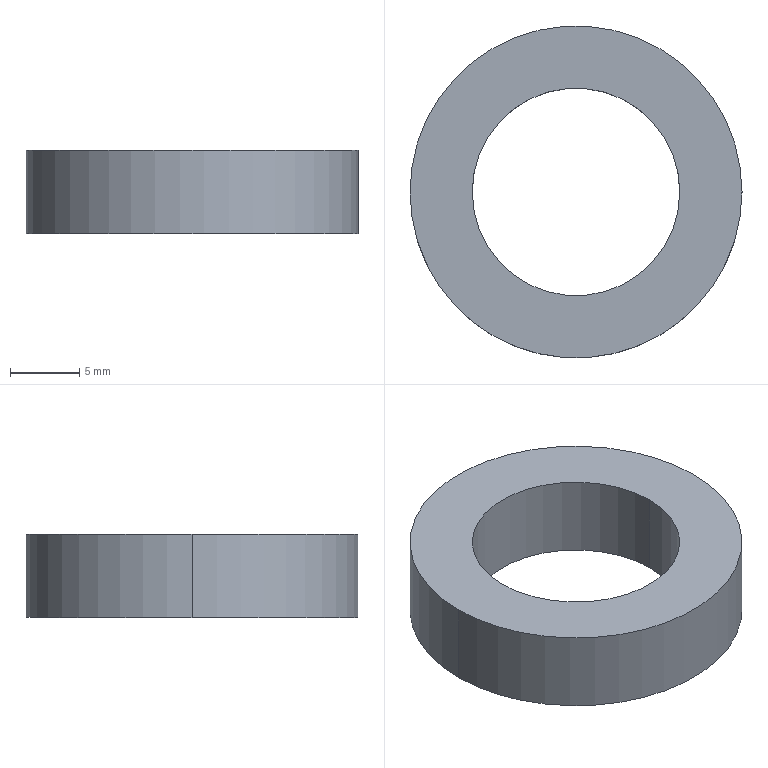Part | STEP file | PN_0016 (stop plate) | 1 solid | 6 faces | box 24 x 24 x 6 mm | volume 1654 mm3 | cylinder 4 | plane 2 | commonest cylinder face diameters 15 x2 24 x2
STEP:
#1=CARTESIAN_POINT('',(0.,0.,0.));
#2=DIRECTION('',(0.,0.,1.));
#3=DIRECTION('',(1.,0.,0.));
#4=AXIS2_PLACEMENT_3D('',#1,#2,#3);
#5=CARTESIAN_POINT('',(-7.5,0.,6.));
#6=VERTEX_POINT('',#5);
#7=CARTESIAN_POINT('',(-7.5,0.,0.));
#8=VERTEX_POINT('',#7);
#9=CARTESIAN_POINT('',(-7.5,0.,6.));
#10=DIRECTION('',(0.,0.,-1.));
#11=VECTOR('',#10,1.);
#12=LINE('',#9,#11);
#13=CARTESIAN_POINT('',(0.,0.,6.));
#14=DIRECTION('',(0.,0.,-1.));
#15=DIRECTION('',(-1.,0.,0.));
#16=AXIS2_PLACEMENT_3D('',#13,#14,#15);
#17=CYLINDRICAL_SURFACE('',#16,7.5);
#18=CARTESIAN_POINT('',(6.283,0.));
#19=DIRECTION('',(0.,1.));
#20=VECTOR('',#19,1.);
#21=LINE('',#18,#20);
#22=(GEOMETRIC_REPRESENTATION_CONTEXT(2)PARAMETRIC_REPRESENTATION_CONTEXT()REPRESENTATION_CONTEXT('',''));
#23=DEFINITIONAL_REPRESENTATION('',(#21),#22);
#24=PCURVE('',#17,#23);
#25=CARTESIAN_POINT('',(0.,0.,6.));
#26=DIRECTION('',(0.,0.,-1.));
#27=DIRECTION('',(-1.,0.,0.));
#28=AXIS2_PLACEMENT_3D('',#25,#26,#27);
#29=CYLINDRICAL_SURFACE('',#28,7.5);
#30=CARTESIAN_POINT('',(0.,0.));
#31=DIRECTION('',(0.,1.));
#32=VECTOR('',#31,1.);
#33=LINE('',#30,#32);
#34=(GEOMETRIC_REPRESENTATION_CONTEXT(2)PARAMETRIC_REPRESENTATION_CONTEXT()REPRESENTATION_CONTEXT('',''));
#35=DEFINITIONAL_REPRESENTATION('',(#33),#34);
#36=PCURVE('',#29,#35);
#37=SURFACE_CURVE('',#12,(#24,#36),.PCURVE_S1.);
#38=EDGE_CURVE('',#6,#8,#37,.T.);
#39=ORIENTED_EDGE('',*,*,#38,.T.);
#40=CARTESIAN_POINT('',(7.5,0.,0.));
#41=VERTEX_POINT('',#40);
#42=CARTESIAN_POINT('',(0.,0.,0.));
#43=DIRECTION('',(0.,0.,1.));
#44=DIRECTION('',(1.,0.,0.));
#45=AXIS2_PLACEMENT_3D('',#42,#43,#44);
#46=CIRCLE('',#45,7.5);
#47=CARTESIAN_POINT('',(9.425,6.));
#48=DIRECTION('',(-1.,0.));
#49=VECTOR('',#48,1.);
#50=LINE('',#47,#49);
#51=(GEOMETRIC_REPRESENTATION_CONTEXT(2)PARAMETRIC_REPRESENTATION_CONTEXT()REPRESENTATION_CONTEXT('',''));
#52=DEFINITIONAL_REPRESENTATION('',(#50),#51);
#53=PCURVE('',#17,#52);
#54=CARTESIAN_POINT('',(0.,0.,0.));
#55=DIRECTION('',(0.,0.,1.));
#56=DIRECTION('',(1.,0.,0.));
#57=AXIS2_PLACEMENT_3D('',#54,#55,#56);
#58=PLANE('',#57);
#59=CARTESIAN_POINT('',(0.,0.));
#60=DIRECTION('',(1.,0.));
#61=AXIS2_PLACEMENT_2D('',#59,#60);
#62=CIRCLE('',#61,7.5);
#63=(GEOMETRIC_REPRESENTATION_CONTEXT(2)PARAMETRIC_REPRESENTATION_CONTEXT()REPRESENTATION_CONTEXT('',''));
#64=DEFINITIONAL_REPRESENTATION('',(#62),#63);
#65=PCURVE('',#58,#64);
#66=SURFACE_CURVE('',#46,(#53,#65),.PCURVE_S1.);
#67=EDGE_CURVE('',#8,#41,#66,.T.);
#68=ORIENTED_EDGE('',*,*,#67,.T.);
#69=CARTESIAN_POINT('',(7.5,0.,6.));
#70=VERTEX_POINT('',#69);
#71=CARTESIAN_POINT('',(7.5,0.,6.));
#72=DIRECTION('',(0.,0.,-1.));
#73=VECTOR('',#72,1.);
#74=LINE('',#71,#73);
#75=CARTESIAN_POINT('',(3.142,0.));
#76=DIRECTION('',(0.,1.));
#77=VECTOR('',#76,1.);
#78=LINE('',#75,#77);
#79=(GEOMETRIC_REPRESENTATION_CONTEXT(2)PARAMETRIC_REPRESENTATION_CONTEXT()REPRESENTATION_CONTEXT('',''));
#80=DEFINITIONAL_REPRESENTATION('',(#78),#79);
#81=PCURVE('',#17,#80);
#82=CARTESIAN_POINT('',(3.142,0.));
#83=DIRECTION('',(0.,1.));
#84=VECTOR('',#83,1.);
#85=LINE('',#82,#84);
#86=(GEOMETRIC_REPRESENTATION_CONTEXT(2)PARAMETRIC_REPRESENTATION_CONTEXT()REPRESENTATION_CONTEXT('',''));
#87=DEFINITIONAL_REPRESENTATION('',(#85),#86);
#88=PCURVE('',#29,#87);
#89=SURFACE_CURVE('',#74,(#81,#88),.PCURVE_S1.);
#90=EDGE_CURVE('',#70,#41,#89,.T.);
#91=ORIENTED_EDGE('',*,*,#90,.F.);
#92=CARTESIAN_POINT('',(0.,0.,6.));
#93=DIRECTION('',(0.,0.,1.));
#94=DIRECTION('',(1.,0.,0.));
#95=AXIS2_PLACEMENT_3D('',#92,#93,#94);
#96=CIRCLE('',#95,7.5);
#97=CARTESIAN_POINT('',(9.425,0.));
#98=DIRECTION('',(-1.,0.));
#99=VECTOR('',#98,1.);
#100=LINE('',#97,#99);
#101=(GEOMETRIC_REPRESENTATION_CONTEXT(2)PARAMETRIC_REPRESENTATION_CONTEXT()REPRESENTATION_CONTEXT('',''));
#102=DEFINITIONAL_REPRESENTATION('',(#100),#101);
#103=PCURVE('',#17,#102);
#104=CARTESIAN_POINT('',(0.,0.,6.));
#105=DIRECTION('',(0.,0.,1.));
#106=DIRECTION('',(1.,0.,0.));
#107=AXIS2_PLACEMENT_3D('',#104,#105,#106);
#108=PLANE('',#107);
#109=CARTESIAN_POINT('',(0.,0.));
#110=DIRECTION('',(1.,0.));
#111=AXIS2_PLACEMENT_2D('',#109,#110);
#112=CIRCLE('',#111,7.5);
#113=(GEOMETRIC_REPRESENTATION_CONTEXT(2)PARAMETRIC_REPRESENTATION_CONTEXT()REPRESENTATION_CONTEXT('',''));
#114=DEFINITIONAL_REPRESENTATION('',(#112),#113);
#115=PCURVE('',#108,#114);
#116=SURFACE_CURVE('',#96,(#103,#115),.PCURVE_S1.);
#117=EDGE_CURVE('',#6,#70,#116,.T.);
#118=ORIENTED_EDGE('',*,*,#117,.F.);
#119=EDGE_LOOP('',(#39,#68,#91,#118));
#120=FACE_BOUND('',#119,.F.);
#121=ADVANCED_FACE('',(#120),#17,.F.);
#122=CARTESIAN_POINT('',(12.,0.,6.));
#123=VERTEX_POINT('',#122);
#124=CARTESIAN_POINT('',(-12.,0.,6.));
#125=VERTEX_POINT('',#124);
#126=CARTESIAN_POINT('',(0.,0.,6.));
#127=DIRECTION('',(0.,0.,1.));
#128=DIRECTION('',(1.,0.,0.));
#129=AXIS2_PLACEMENT_3D('',#126,#127,#128);
#130=CIRCLE('',#129,12.);
#131=CARTESIAN_POINT('',(0.,0.,6.));
#132=DIRECTION('',(0.,0.,-1.));
#133=DIRECTION('',(-1.,0.,0.));
#134=AXIS2_PLACEMENT_3D('',#131,#132,#133);
#135=CYLINDRICAL_SURFACE('',#134,12.);
#136=CARTESIAN_POINT('',(3.142,0.));
#137=DIRECTION('',(-1.,0.));
#138=VECTOR('',#137,1.);
#139=LINE('',#136,#138);
#140=(GEOMETRIC_REPRESENTATION_CONTEXT(2)PARAMETRIC_REPRESENTATION_CONTEXT()REPRESENTATION_CONTEXT('',''));
#141=DEFINITIONAL_REPRESENTATION('',(#139),#140);
#142=PCURVE('',#135,#141);
#143=CARTESIAN_POINT('',(0.,0.));
#144=DIRECTION('',(1.,0.));
#145=AXIS2_PLACEMENT_2D('',#143,#144);
#146=CIRCLE('',#145,12.);
#147=(GEOMETRIC_REPRESENTATION_CONTEXT(2)PARAMETRIC_REPRESENTATION_CONTEXT()REPRESENTATION_CONTEXT('',''));
#148=DEFINITIONAL_REPRESENTATION('',(#146),#147);
#149=PCURVE('',#108,#148);
#150=SURFACE_CURVE('',#130,(#142,#149),.PCURVE_S1.);
#151=EDGE_CURVE('',#123,#125,#150,.T.);
#152=ORIENTED_EDGE('',*,*,#151,.F.);
#153=CARTESIAN_POINT('',(12.,0.,0.));
#154=VERTEX_POINT('',#153);
#155=CARTESIAN_POINT('',(12.,0.,6.));
#156=DIRECTION('',(0.,0.,-1.));
#157=VECTOR('',#156,1.);
#158=LINE('',#155,#157);
#159=CARTESIAN_POINT('',(3.142,0.));
#160=DIRECTION('',(0.,1.));
#161=VECTOR('',#160,1.);
#162=LINE('',#159,#161);
#163=(GEOMETRIC_REPRESENTATION_CONTEXT(2)PARAMETRIC_REPRESENTATION_CONTEXT()REPRESENTATION_CONTEXT('',''));
#164=DEFINITIONAL_REPRESENTATION('',(#162),#163);
#165=PCURVE('',#135,#164);
#166=CARTESIAN_POINT('',(0.,0.,6.));
#167=DIRECTION('',(0.,0.,-1.));
#168=DIRECTION('',(-1.,0.,0.));
#169=AXIS2_PLACEMENT_3D('',#166,#167,#168);
#170=CYLINDRICAL_SURFACE('',#169,12.);
#171=CARTESIAN_POINT('',(3.142,0.));
#172=DIRECTION('',(0.,1.));
#173=VECTOR('',#172,1.);
#174=LINE('',#171,#173);
#175=(GEOMETRIC_REPRESENTATION_CONTEXT(2)PARAMETRIC_REPRESENTATION_CONTEXT()REPRESENTATION_CONTEXT('',''));
#176=DEFINITIONAL_REPRESENTATION('',(#174),#175);
#177=PCURVE('',#170,#176);
#178=SURFACE_CURVE('',#158,(#165,#177),.PCURVE_S1.);
#179=EDGE_CURVE('',#123,#154,#178,.T.);
#180=ORIENTED_EDGE('',*,*,#179,.T.);
#181=CARTESIAN_POINT('',(-12.,0.,0.));
#182=VERTEX_POINT('',#181);
#183=CARTESIAN_POINT('',(0.,0.,0.));
#184=DIRECTION('',(0.,0.,1.));
#185=DIRECTION('',(1.,0.,0.));
#186=AXIS2_PLACEMENT_3D('',#183,#184,#185);
#187=CIRCLE('',#186,12.);
#188=CARTESIAN_POINT('',(3.142,6.));
#189=DIRECTION('',(-1.,0.));
#190=VECTOR('',#189,1.);
#191=LINE('',#188,#190);
#192=(GEOMETRIC_REPRESENTATION_CONTEXT(2)PARAMETRIC_REPRESENTATION_CONTEXT()REPRESENTATION_CONTEXT('',''));
#193=DEFINITIONAL_REPRESENTATION('',(#191),#192);
#194=PCURVE('',#135,#193);
#195=CARTESIAN_POINT('',(0.,0.));
#196=DIRECTION('',(1.,0.));
#197=AXIS2_PLACEMENT_2D('',#195,#196);
#198=CIRCLE('',#197,12.);
#199=(GEOMETRIC_REPRESENTATION_CONTEXT(2)PARAMETRIC_REPRESENTATION_CONTEXT()REPRESENTATION_CONTEXT('',''));
#200=DEFINITIONAL_REPRESENTATION('',(#198),#199);
#201=PCURVE('',#58,#200);
#202=SURFACE_CURVE('',#187,(#194,#201),.PCURVE_S1.);
#203=EDGE_CURVE('',#154,#182,#202,.T.);
#204=ORIENTED_EDGE('',*,*,#203,.T.);
#205=CARTESIAN_POINT('',(-12.,0.,6.));
#206=DIRECTION('',(0.,0.,-1.));
#207=VECTOR('',#206,1.);
#208=LINE('',#205,#207);
#209=CARTESIAN_POINT('',(0.,0.));
#210=DIRECTION('',(0.,1.));
#211=VECTOR('',#210,1.);
#212=LINE('',#209,#211);
#213=(GEOMETRIC_REPRESENTATION_CONTEXT(2)PARAMETRIC_REPRESENTATION_CONTEXT()REPRESENTATION_CONTEXT('',''));
#214=DEFINITIONAL_REPRESENTATION('',(#212),#213);
#215=PCURVE('',#135,#214);
#216=CARTESIAN_POINT('',(6.283,0.));
#217=DIRECTION('',(0.,1.));
#218=VECTOR('',#217,1.);
#219=LINE('',#216,#218);
#220=(GEOMETRIC_REPRESENTATION_CONTEXT(2)PARAMETRIC_REPRESENTATION_CONTEXT()REPRESENTATION_CONTEXT('',''));
#221=DEFINITIONAL_REPRESENTATION('',(#219),#220);
#222=PCURVE('',#170,#221);
#223=SURFACE_CURVE('',#208,(#215,#222),.PCURVE_S1.);
#224=EDGE_CURVE('',#125,#182,#223,.T.);
#225=ORIENTED_EDGE('',*,*,#224,.F.);
#226=EDGE_LOOP('',(#152,#180,#204,#225));
#227=FACE_BOUND('',#226,.T.);
#228=ADVANCED_FACE('',(#227),#135,.T.);
#229=CARTESIAN_POINT('',(0.,0.,6.));
#230=DIRECTION('',(0.,0.,1.));
#231=DIRECTION('',(1.,0.,0.));
#232=AXIS2_PLACEMENT_3D('',#229,#230,#231);
#233=CIRCLE('',#232,12.);
#234=CARTESIAN_POINT('',(0.,0.));
#235=DIRECTION('',(1.,0.));
#236=AXIS2_PLACEMENT_2D('',#234,#235);
#237=CIRCLE('',#236,12.);
#238=(GEOMETRIC_REPRESENTATION_CONTEXT(2)PARAMETRIC_REPRESENTATION_CONTEXT()REPRESENTATION_CONTEXT('',''));
#239=DEFINITIONAL_REPRESENTATION('',(#237),#238);
#240=PCURVE('',#108,#239);
#241=CARTESIAN_POINT('',(9.425,0.));
#242=DIRECTION('',(-1.,0.));
#243=VECTOR('',#242,1.);
#244=LINE('',#241,#243);
#245=(GEOMETRIC_REPRESENTATION_CONTEXT(2)PARAMETRIC_REPRESENTATION_CONTEXT()REPRESENTATION_CONTEXT('',''));
#246=DEFINITIONAL_REPRESENTATION('',(#244),#245);
#247=PCURVE('',#170,#246);
#248=SURFACE_CURVE('',#233,(#240,#247),.PCURVE_S1.);
#249=EDGE_CURVE('',#125,#123,#248,.T.);
#250=ORIENTED_EDGE('',*,*,#249,.T.);
#251=ORIENTED_EDGE('',*,*,#151,.T.);
#252=EDGE_LOOP('',(#250,#251));
#253=FACE_BOUND('',#252,.T.);
#254=ORIENTED_EDGE('',*,*,#117,.F.);
#255=CARTESIAN_POINT('',(0.,0.,6.));
#256=DIRECTION('',(0.,0.,1.));
#257=DIRECTION('',(1.,0.,0.));
#258=AXIS2_PLACEMENT_3D('',#255,#256,#257);
#259=CIRCLE('',#258,7.5);
#260=CARTESIAN_POINT('',(0.,0.));
#261=DIRECTION('',(1.,0.));
#262=AXIS2_PLACEMENT_2D('',#260,#261);
#263=CIRCLE('',#262,7.5);
#264=(GEOMETRIC_REPRESENTATION_CONTEXT(2)PARAMETRIC_REPRESENTATION_CONTEXT()REPRESENTATION_CONTEXT('',''));
#265=DEFINITIONAL_REPRESENTATION('',(#263),#264);
#266=PCURVE('',#108,#265);
#267=CARTESIAN_POINT('',(3.142,0.));
#268=DIRECTION('',(-1.,0.));
#269=VECTOR('',#268,1.);
#270=LINE('',#267,#269);
#271=(GEOMETRIC_REPRESENTATION_CONTEXT(2)PARAMETRIC_REPRESENTATION_CONTEXT()REPRESENTATION_CONTEXT('',''));
#272=DEFINITIONAL_REPRESENTATION('',(#270),#271);
#273=PCURVE('',#29,#272);
#274=SURFACE_CURVE('',#259,(#266,#273),.PCURVE_S1.);
#275=EDGE_CURVE('',#70,#6,#274,.T.);
#276=ORIENTED_EDGE('',*,*,#275,.F.);
#277=EDGE_LOOP('',(#254,#276));
#278=FACE_BOUND('',#277,.T.);
#279=ADVANCED_FACE('',(#253,#278),#108,.T.);
#280=CARTESIAN_POINT('',(0.,0.,0.));
#281=DIRECTION('',(0.,0.,1.));
#282=DIRECTION('',(1.,0.,0.));
#283=AXIS2_PLACEMENT_3D('',#280,#281,#282);
#284=CIRCLE('',#283,12.);
#285=CARTESIAN_POINT('',(0.,0.));
#286=DIRECTION('',(1.,0.));
#287=AXIS2_PLACEMENT_2D('',#285,#286);
#288=CIRCLE('',#287,12.);
#289=(GEOMETRIC_REPRESENTATION_CONTEXT(2)PARAMETRIC_REPRESENTATION_CONTEXT()REPRESENTATION_CONTEXT('',''));
#290=DEFINITIONAL_REPRESENTATION('',(#288),#289);
#291=PCURVE('',#58,#290);
#292=CARTESIAN_POINT('',(9.425,6.));
#293=DIRECTION('',(-1.,0.));
#294=VECTOR('',#293,1.);
#295=LINE('',#292,#294);
#296=(GEOMETRIC_REPRESENTATION_CONTEXT(2)PARAMETRIC_REPRESENTATION_CONTEXT()REPRESENTATION_CONTEXT('',''));
#297=DEFINITIONAL_REPRESENTATION('',(#295),#296);
#298=PCURVE('',#170,#297);
#299=SURFACE_CURVE('',#284,(#291,#298),.PCURVE_S1.);
#300=EDGE_CURVE('',#182,#154,#299,.T.);
#301=ORIENTED_EDGE('',*,*,#300,.F.);
#302=ORIENTED_EDGE('',*,*,#203,.F.);
#303=EDGE_LOOP('',(#301,#302));
#304=FACE_BOUND('',#303,.T.);
#305=ORIENTED_EDGE('',*,*,#67,.T.);
#306=CARTESIAN_POINT('',(0.,0.,0.));
#307=DIRECTION('',(0.,0.,1.));
#308=DIRECTION('',(1.,0.,0.));
#309=AXIS2_PLACEMENT_3D('',#306,#307,#308);
#310=CIRCLE('',#309,7.5);
#311=CARTESIAN_POINT('',(0.,0.));
#312=DIRECTION('',(1.,0.));
#313=AXIS2_PLACEMENT_2D('',#311,#312);
#314=CIRCLE('',#313,7.5);
#315=(GEOMETRIC_REPRESENTATION_CONTEXT(2)PARAMETRIC_REPRESENTATION_CONTEXT()REPRESENTATION_CONTEXT('',''));
#316=DEFINITIONAL_REPRESENTATION('',(#314),#315);
#317=PCURVE('',#58,#316);
#318=CARTESIAN_POINT('',(3.142,6.));
#319=DIRECTION('',(-1.,0.));
#320=VECTOR('',#319,1.);
#321=LINE('',#318,#320);
#322=(GEOMETRIC_REPRESENTATION_CONTEXT(2)PARAMETRIC_REPRESENTATION_CONTEXT()REPRESENTATION_CONTEXT('',''));
#323=DEFINITIONAL_REPRESENTATION('',(#321),#322);
#324=PCURVE('',#29,#323);
#325=SURFACE_CURVE('',#310,(#317,#324),.PCURVE_S1.);
#326=EDGE_CURVE('',#41,#8,#325,.T.);
#327=ORIENTED_EDGE('',*,*,#326,.T.);
#328=EDGE_LOOP('',(#305,#327));
#329=FACE_BOUND('',#328,.T.);
#330=ADVANCED_FACE('',(#304,#329),#58,.F.);
#331=ORIENTED_EDGE('',*,*,#179,.F.);
#332=ORIENTED_EDGE('',*,*,#249,.F.);
#333=ORIENTED_EDGE('',*,*,#224,.T.);
#334=ORIENTED_EDGE('',*,*,#300,.T.);
#335=EDGE_LOOP('',(#331,#332,#333,#334));
#336=FACE_BOUND('',#335,.T.);
#337=ADVANCED_FACE('',(#336),#170,.T.);
#338=ORIENTED_EDGE('',*,*,#326,.T.);
#339=ORIENTED_EDGE('',*,*,#38,.F.);
#340=ORIENTED_EDGE('',*,*,#275,.F.);
#341=ORIENTED_EDGE('',*,*,#90,.T.);
#342=EDGE_LOOP('',(#338,#339,#340,#341));
#343=FACE_BOUND('',#342,.F.);
#344=ADVANCED_FACE('',(#343),#29,.F.);
#345=CLOSED_SHELL('',(#121,#228,#279,#330,#337,#344));
#346=MANIFOLD_SOLID_BREP('',#345);
#347=(LENGTH_UNIT()NAMED_UNIT(*)SI_UNIT(.MILLI.,.METRE.));
#348=UNCERTAINTY_MEASURE_WITH_UNIT(LENGTH_MEASURE(0.0000001),#347,'','');
#349=(NAMED_UNIT(*)PLANE_ANGLE_UNIT()SI_UNIT($,.RADIAN.));
#350=(NAMED_UNIT(*)SI_UNIT($,.STERADIAN.)SOLID_ANGLE_UNIT());
#351=(GEOMETRIC_REPRESENTATION_CONTEXT(3)GLOBAL_UNCERTAINTY_ASSIGNED_CONTEXT((#348))GLOBAL_UNIT_ASSIGNED_CONTEXT((#347,#349,#350))REPRESENTATION_CONTEXT('',''));
#352=ADVANCED_BREP_SHAPE_REPRESENTATION('',(#4,#346),#351);